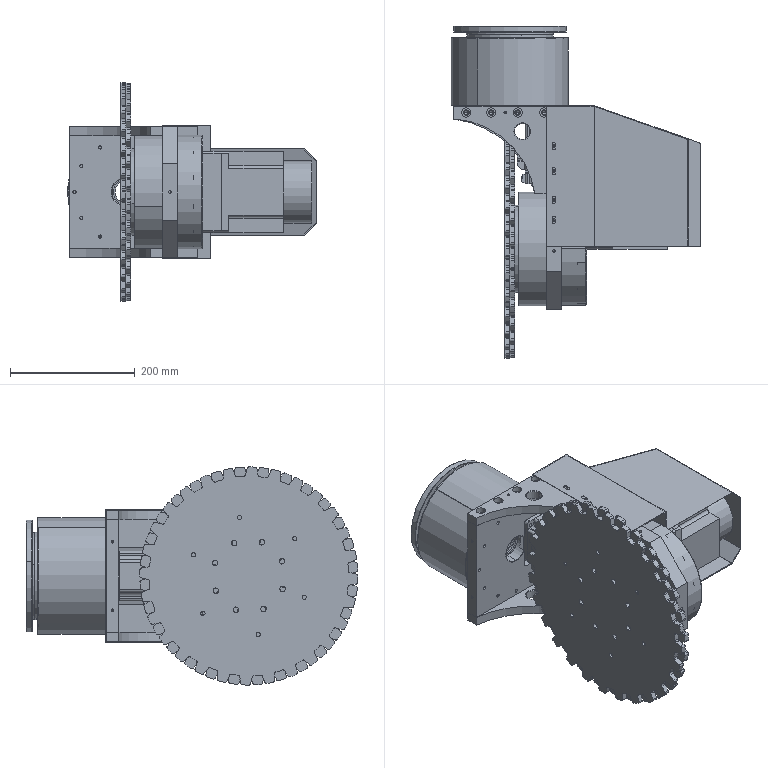Part | SolidWorks | features InContextFeatHolder 38, CompositeCurve 7 | 30 solids | 2404 faces | box 400 x 532.5 x 350 mm | volume 11036293 mm3 | cylinder 1510 | plane 593 | cone 273 | torus 26 | sphere 2 | commonest cylinder face diameters 6 x306 5 x117 9 x113 12.5 x108 6.6 x94 6.8 x92